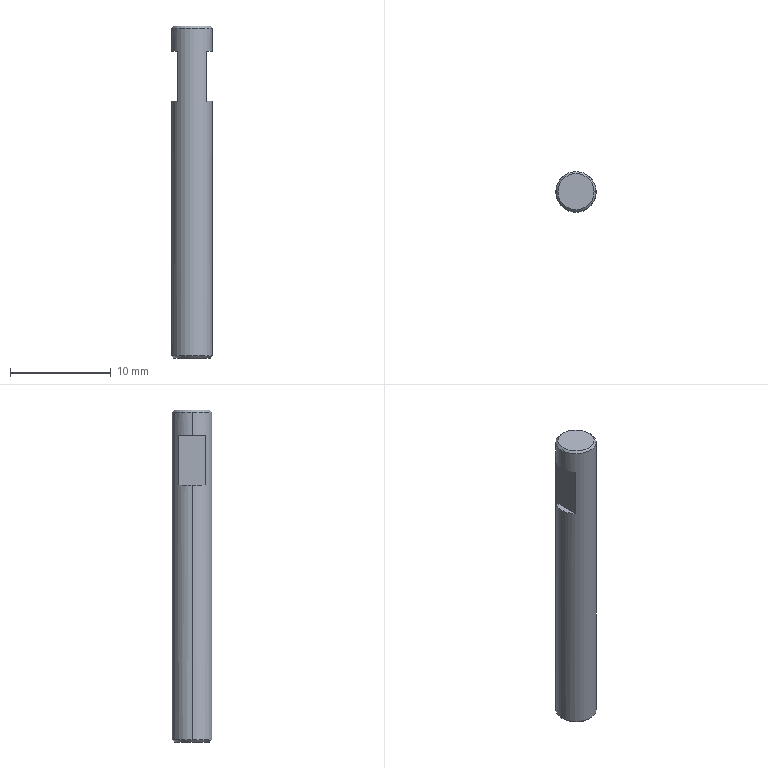Part | SolidWorks | features BaseBody 1, Chamfer 1 | 1 solid | 18 faces | box 4 x 4 x 33 mm | volume 382.151 mm3 | plane 8 | cone 6 | cylinder 4 | commonest cylinder face diameters 2.05 x2 4 x2
STEP:
#1=CARTESIAN_POINT('',(1.8,0.,16.5));
#2=VERTEX_POINT('',#1);
#3=CARTESIAN_POINT('',(-1.8,0.,16.5));
#4=VERTEX_POINT('',#3);
#5=CARTESIAN_POINT('',(0.,0.,16.5));
#6=DIRECTION('',(0.,0.,1.));
#7=DIRECTION('',(1.,0.,0.));
#8=AXIS2_PLACEMENT_3D('',#5,#6,#7);
#9=CIRCLE('',#8,1.8);
#10=EDGE_CURVE('',#2,#4,#9,.T.);
#11=ORIENTED_EDGE('',*,*,#10,.F.);
#12=CARTESIAN_POINT('',(2.,0.,16.3));
#13=VERTEX_POINT('',#12);
#14=CARTESIAN_POINT('',(2.,0.,16.3));
#15=DIRECTION('',(0.7071,0.,-0.7071));
#16=VECTOR('',#15,1000.);
#17=LINE('',#14,#16);
#18=EDGE_CURVE('',#2,#13,#17,.T.);
#19=ORIENTED_EDGE('',*,*,#18,.T.);
#20=CARTESIAN_POINT('',(-2.,0.,16.3));
#21=VERTEX_POINT('',#20);
#22=CARTESIAN_POINT('',(0.,0.,16.3));
#23=DIRECTION('',(0.,0.,-1.));
#24=DIRECTION('',(1.,0.,0.));
#25=AXIS2_PLACEMENT_3D('',#22,#23,#24);
#26=CIRCLE('',#25,2.);
#27=EDGE_CURVE('',#21,#13,#26,.T.);
#28=ORIENTED_EDGE('',*,*,#27,.F.);
#29=CARTESIAN_POINT('',(-2.,0.,16.3));
#30=DIRECTION('',(-0.7071,0.,-0.7071));
#31=VECTOR('',#30,1000.);
#32=LINE('',#29,#31);
#33=EDGE_CURVE('',#4,#21,#32,.T.);
#34=ORIENTED_EDGE('',*,*,#33,.F.);
#35=EDGE_LOOP('',(#11,#19,#28,#34));
#36=FACE_OUTER_BOUND('',#35,.T.);
#37=CARTESIAN_POINT('',(0.,0.,16.3));
#38=DIRECTION('',(0.,0.,-1.));
#39=DIRECTION('',(-1.,0.,0.));
#40=AXIS2_PLACEMENT_3D('',#37,#38,#39);
#41=CONICAL_SURFACE('',#40,2.,0.7854);
#42=ADVANCED_FACE('',(#36),#41,.T.);
#43=CARTESIAN_POINT('',(-1.8,0.,-16.5));
#44=VERTEX_POINT('',#43);
#45=CARTESIAN_POINT('',(1.8,0.,-16.5));
#46=VERTEX_POINT('',#45);
#47=CARTESIAN_POINT('',(0.,0.,-16.5));
#48=DIRECTION('',(0.,0.,-1.));
#49=DIRECTION('',(1.,0.,0.));
#50=AXIS2_PLACEMENT_3D('',#47,#48,#49);
#51=CIRCLE('',#50,1.8);
#52=EDGE_CURVE('',#44,#46,#51,.T.);
#53=ORIENTED_EDGE('',*,*,#52,.F.);
#54=CARTESIAN_POINT('',(-2.,0.,-16.3));
#55=VERTEX_POINT('',#54);
#56=CARTESIAN_POINT('',(-2.,0.,-16.3));
#57=DIRECTION('',(-0.7071,0.,0.7071));
#58=VECTOR('',#57,1000.);
#59=LINE('',#56,#58);
#60=EDGE_CURVE('',#44,#55,#59,.T.);
#61=ORIENTED_EDGE('',*,*,#60,.T.);
#62=CARTESIAN_POINT('',(2.,0.,-16.3));
#63=VERTEX_POINT('',#62);
#64=CARTESIAN_POINT('',(0.,0.,-16.3));
#65=DIRECTION('',(0.,0.,1.));
#66=DIRECTION('',(1.,0.,0.));
#67=AXIS2_PLACEMENT_3D('',#64,#65,#66);
#68=CIRCLE('',#67,2.);
#69=EDGE_CURVE('',#63,#55,#68,.T.);
#70=ORIENTED_EDGE('',*,*,#69,.F.);
#71=CARTESIAN_POINT('',(2.,0.,-16.3));
#72=DIRECTION('',(0.7071,0.,0.7071));
#73=VECTOR('',#72,1000.);
#74=LINE('',#71,#73);
#75=EDGE_CURVE('',#46,#63,#74,.T.);
#76=ORIENTED_EDGE('',*,*,#75,.F.);
#77=EDGE_LOOP('',(#53,#61,#70,#76));
#78=FACE_OUTER_BOUND('',#77,.T.);
#79=CARTESIAN_POINT('',(0.,0.,-16.3));
#80=DIRECTION('',(0.,0.,1.));
#81=DIRECTION('',(1.,0.,0.));
#82=AXIS2_PLACEMENT_3D('',#79,#80,#81);
#83=CONICAL_SURFACE('',#82,2.,0.7854);
#84=ADVANCED_FACE('',(#78),#83,.T.);
#85=ORIENTED_EDGE('',*,*,#27,.T.);
#86=CARTESIAN_POINT('',(2.,0.,14.));
#87=VERTEX_POINT('',#86);
#88=CARTESIAN_POINT('',(2.,0.,16.5));
#89=DIRECTION('',(0.,0.,-1.));
#90=VECTOR('',#89,1000.);
#91=LINE('',#88,#90);
#92=EDGE_CURVE('',#13,#87,#91,.T.);
#93=ORIENTED_EDGE('',*,*,#92,.T.);
#94=CARTESIAN_POINT('',(1.45,1.377,14.));
#95=VERTEX_POINT('',#94);
#96=CARTESIAN_POINT('',(0.,0.,14.));
#97=DIRECTION('',(0.,0.,1.));
#98=DIRECTION('',(-1.,0.,0.));
#99=AXIS2_PLACEMENT_3D('',#96,#97,#98);
#100=CIRCLE('',#99,2.);
#101=EDGE_CURVE('',#87,#95,#100,.T.);
#102=ORIENTED_EDGE('',*,*,#101,.T.);
#103=CARTESIAN_POINT('',(1.45,1.377,9.));
#104=VERTEX_POINT('',#103);
#105=CARTESIAN_POINT('',(1.45,1.377,16.5));
#106=DIRECTION('',(0.,0.,-1.));
#107=VECTOR('',#106,1000.);
#108=LINE('',#105,#107);
#109=EDGE_CURVE('',#95,#104,#108,.T.);
#110=ORIENTED_EDGE('',*,*,#109,.T.);
#111=CARTESIAN_POINT('',(2.,0.,9.));
#112=VERTEX_POINT('',#111);
#113=CARTESIAN_POINT('',(0.,0.,9.));
#114=DIRECTION('',(0.,0.,-1.));
#115=DIRECTION('',(-1.,0.,0.));
#116=AXIS2_PLACEMENT_3D('',#113,#114,#115);
#117=CIRCLE('',#116,2.);
#118=EDGE_CURVE('',#104,#112,#117,.T.);
#119=ORIENTED_EDGE('',*,*,#118,.T.);
#120=CARTESIAN_POINT('',(2.,0.,16.5));
#121=DIRECTION('',(0.,0.,-1.));
#122=VECTOR('',#121,1000.);
#123=LINE('',#120,#122);
#124=EDGE_CURVE('',#112,#63,#123,.T.);
#125=ORIENTED_EDGE('',*,*,#124,.T.);
#126=ORIENTED_EDGE('',*,*,#69,.T.);
#127=CARTESIAN_POINT('',(-2.,0.,9.));
#128=VERTEX_POINT('',#127);
#129=CARTESIAN_POINT('',(-2.,0.,16.5));
#130=DIRECTION('',(0.,0.,-1.));
#131=VECTOR('',#130,1000.);
#132=LINE('',#129,#131);
#133=EDGE_CURVE('',#128,#55,#132,.T.);
#134=ORIENTED_EDGE('',*,*,#133,.F.);
#135=CARTESIAN_POINT('',(-1.45,1.377,9.));
#136=VERTEX_POINT('',#135);
#137=CARTESIAN_POINT('',(0.,0.,9.));
#138=DIRECTION('',(0.,0.,-1.));
#139=DIRECTION('',(-1.,0.,0.));
#140=AXIS2_PLACEMENT_3D('',#137,#138,#139);
#141=CIRCLE('',#140,2.);
#142=EDGE_CURVE('',#128,#136,#141,.T.);
#143=ORIENTED_EDGE('',*,*,#142,.T.);
#144=CARTESIAN_POINT('',(-1.45,1.377,14.));
#145=VERTEX_POINT('',#144);
#146=CARTESIAN_POINT('',(-1.45,1.377,16.5));
#147=DIRECTION('',(0.,0.,1.));
#148=VECTOR('',#147,1000.);
#149=LINE('',#146,#148);
#150=EDGE_CURVE('',#136,#145,#149,.T.);
#151=ORIENTED_EDGE('',*,*,#150,.T.);
#152=CARTESIAN_POINT('',(-2.,0.,14.));
#153=VERTEX_POINT('',#152);
#154=CARTESIAN_POINT('',(0.,0.,14.));
#155=DIRECTION('',(0.,0.,1.));
#156=DIRECTION('',(-1.,0.,0.));
#157=AXIS2_PLACEMENT_3D('',#154,#155,#156);
#158=CIRCLE('',#157,2.);
#159=EDGE_CURVE('',#145,#153,#158,.T.);
#160=ORIENTED_EDGE('',*,*,#159,.T.);
#161=CARTESIAN_POINT('',(-2.,0.,16.5));
#162=DIRECTION('',(0.,0.,-1.));
#163=VECTOR('',#162,1000.);
#164=LINE('',#161,#163);
#165=EDGE_CURVE('',#21,#153,#164,.T.);
#166=ORIENTED_EDGE('',*,*,#165,.F.);
#167=EDGE_LOOP('',(#85,#93,#102,#110,#119,#125,#126,#134,#143,#151,#160,#166));
#168=FACE_OUTER_BOUND('',#167,.T.);
#169=CARTESIAN_POINT('',(0.,0.,16.5));
#170=DIRECTION('',(0.,0.,-1.));
#171=DIRECTION('',(-1.,0.,0.));
#172=AXIS2_PLACEMENT_3D('',#169,#170,#171);
#173=CYLINDRICAL_SURFACE('',#172,2.);
#174=ADVANCED_FACE('',(#168),#173,.T.);
#175=CARTESIAN_POINT('',(1.025,0.,-10.15));
#176=VERTEX_POINT('',#175);
#177=CARTESIAN_POINT('',(-1.025,0.,-10.15));
#178=VERTEX_POINT('',#177);
#179=CARTESIAN_POINT('',(0.,0.,-10.15));
#180=DIRECTION('',(0.,0.,-1.));
#181=DIRECTION('',(-1.,0.,0.));
#182=AXIS2_PLACEMENT_3D('',#179,#180,#181);
#183=CIRCLE('',#182,1.025);
#184=EDGE_CURVE('',#176,#178,#183,.T.);
#185=ORIENTED_EDGE('',*,*,#184,.F.);
#186=CARTESIAN_POINT('',(1.025,0.,-16.5));
#187=VERTEX_POINT('',#186);
#188=CARTESIAN_POINT('',(1.025,0.,-16.5));
#189=DIRECTION('',(0.,0.,-1.));
#190=VECTOR('',#189,1000.);
#191=LINE('',#188,#190);
#192=EDGE_CURVE('',#176,#187,#191,.T.);
#193=ORIENTED_EDGE('',*,*,#192,.T.);
#194=CARTESIAN_POINT('',(-1.025,0.,-16.5));
#195=VERTEX_POINT('',#194);
#196=CARTESIAN_POINT('',(0.,0.,-16.5));
#197=DIRECTION('',(0.,0.,-1.));
#198=DIRECTION('',(-1.,0.,0.));
#199=AXIS2_PLACEMENT_3D('',#196,#197,#198);
#200=CIRCLE('',#199,1.025);
#201=EDGE_CURVE('',#187,#195,#200,.T.);
#202=ORIENTED_EDGE('',*,*,#201,.T.);
#203=CARTESIAN_POINT('',(-1.025,0.,-16.5));
#204=DIRECTION('',(0.,0.,-1.));
#205=VECTOR('',#204,1000.);
#206=LINE('',#203,#205);
#207=EDGE_CURVE('',#178,#195,#206,.T.);
#208=ORIENTED_EDGE('',*,*,#207,.F.);
#209=EDGE_LOOP('',(#185,#193,#202,#208));
#210=FACE_OUTER_BOUND('',#209,.T.);
#211=CARTESIAN_POINT('',(0.,0.,-16.5));
#212=DIRECTION('',(0.,0.,-1.));
#213=DIRECTION('',(-1.,0.,0.));
#214=AXIS2_PLACEMENT_3D('',#211,#212,#213);
#215=CYLINDRICAL_SURFACE('',#214,1.025);
#216=ADVANCED_FACE('',(#210),#215,.F.);
#217=CARTESIAN_POINT('',(0.,0.,-9.534));
#218=VERTEX_POINT('',#217);
#219=CARTESIAN_POINT('',(-1.025,0.,-10.15));
#220=DIRECTION('',(-0.8572,0.,-0.515));
#221=VECTOR('',#220,1000.);
#222=LINE('',#219,#221);
#223=EDGE_CURVE('',#218,#178,#222,.T.);
#224=ORIENTED_EDGE('',*,*,#223,.F.);
#225=CARTESIAN_POINT('',(1.025,0.,-10.15));
#226=DIRECTION('',(0.8572,0.,-0.515));
#227=VECTOR('',#226,1000.);
#228=LINE('',#225,#227);
#229=EDGE_CURVE('',#218,#176,#228,.T.);
#230=ORIENTED_EDGE('',*,*,#229,.T.);
#231=ORIENTED_EDGE('',*,*,#184,.T.);
#232=EDGE_LOOP('',(#224,#230,#231));
#233=FACE_OUTER_BOUND('',#232,.T.);
#234=CARTESIAN_POINT('',(0.,0.,-10.15));
#235=DIRECTION('',(0.,0.,-1.));
#236=DIRECTION('',(-1.,0.,0.));
#237=AXIS2_PLACEMENT_3D('',#234,#235,#236);
#238=CONICAL_SURFACE('',#237,1.025,1.03);
#239=ADVANCED_FACE('',(#233),#238,.F.);
#240=ORIENTED_EDGE('',*,*,#92,.F.);
#241=CARTESIAN_POINT('',(0.,0.,16.3));
#242=DIRECTION('',(0.,0.,-1.));
#243=DIRECTION('',(1.,0.,0.));
#244=AXIS2_PLACEMENT_3D('',#241,#242,#243);
#245=CIRCLE('',#244,2.);
#246=EDGE_CURVE('',#13,#21,#245,.T.);
#247=ORIENTED_EDGE('',*,*,#246,.T.);
#248=ORIENTED_EDGE('',*,*,#165,.T.);
#249=CARTESIAN_POINT('',(-1.45,-1.377,14.));
#250=VERTEX_POINT('',#249);
#251=CARTESIAN_POINT('',(0.,0.,14.));
#252=DIRECTION('',(0.,0.,1.));
#253=DIRECTION('',(-1.,0.,0.));
#254=AXIS2_PLACEMENT_3D('',#251,#252,#253);
#255=CIRCLE('',#254,2.);
#256=EDGE_CURVE('',#153,#250,#255,.T.);
#257=ORIENTED_EDGE('',*,*,#256,.T.);
#258=CARTESIAN_POINT('',(-1.45,-1.377,9.));
#259=VERTEX_POINT('',#258);
#260=CARTESIAN_POINT('',(-1.45,-1.377,16.5));
#261=DIRECTION('',(0.,0.,-1.));
#262=VECTOR('',#261,1000.);
#263=LINE('',#260,#262);
#264=EDGE_CURVE('',#250,#259,#263,.T.);
#265=ORIENTED_EDGE('',*,*,#264,.T.);
#266=CARTESIAN_POINT('',(0.,0.,9.));
#267=DIRECTION('',(0.,0.,-1.));
#268=DIRECTION('',(-1.,0.,0.));
#269=AXIS2_PLACEMENT_3D('',#266,#267,#268);
#270=CIRCLE('',#269,2.);
#271=EDGE_CURVE('',#259,#128,#270,.T.);
#272=ORIENTED_EDGE('',*,*,#271,.T.);
#273=ORIENTED_EDGE('',*,*,#133,.T.);
#274=CARTESIAN_POINT('',(0.,0.,-16.3));
#275=DIRECTION('',(0.,0.,1.));
#276=DIRECTION('',(1.,0.,0.));
#277=AXIS2_PLACEMENT_3D('',#274,#275,#276);
#278=CIRCLE('',#277,2.);
#279=EDGE_CURVE('',#55,#63,#278,.T.);
#280=ORIENTED_EDGE('',*,*,#279,.T.);
#281=ORIENTED_EDGE('',*,*,#124,.F.);
#282=CARTESIAN_POINT('',(1.45,-1.377,9.));
#283=VERTEX_POINT('',#282);
#284=CARTESIAN_POINT('',(0.,0.,9.));
#285=DIRECTION('',(0.,0.,-1.));
#286=DIRECTION('',(-1.,0.,0.));
#287=AXIS2_PLACEMENT_3D('',#284,#285,#286);
#288=CIRCLE('',#287,2.);
#289=EDGE_CURVE('',#112,#283,#288,.T.);
#290=ORIENTED_EDGE('',*,*,#289,.T.);
#291=CARTESIAN_POINT('',(1.45,-1.377,14.));
#292=VERTEX_POINT('',#291);
#293=CARTESIAN_POINT('',(1.45,-1.377,16.5));
#294=DIRECTION('',(0.,0.,1.));
#295=VECTOR('',#294,1000.);
#296=LINE('',#293,#295);
#297=EDGE_CURVE('',#283,#292,#296,.T.);
#298=ORIENTED_EDGE('',*,*,#297,.T.);
#299=CARTESIAN_POINT('',(0.,0.,14.));
#300=DIRECTION('',(0.,0.,1.));
#301=DIRECTION('',(-1.,0.,0.));
#302=AXIS2_PLACEMENT_3D('',#299,#300,#301);
#303=CIRCLE('',#302,2.);
#304=EDGE_CURVE('',#292,#87,#303,.T.);
#305=ORIENTED_EDGE('',*,*,#304,.T.);
#306=EDGE_LOOP('',(#240,#247,#248,#257,#265,#272,#273,#280,#281,#290,#298,#305));
#307=FACE_OUTER_BOUND('',#306,.T.);
#308=CARTESIAN_POINT('',(0.,0.,16.5));
#309=DIRECTION('',(0.,0.,-1.));
#310=DIRECTION('',(-1.,0.,0.));
#311=AXIS2_PLACEMENT_3D('',#308,#309,#310);
#312=CYLINDRICAL_SURFACE('',#311,2.);
#313=ADVANCED_FACE('',(#307),#312,.T.);
#314=CARTESIAN_POINT('',(-1.45,-2.,14.));
#315=DIRECTION('',(0.,1.,0.));
#316=VECTOR('',#315,1000.);
#317=LINE('',#314,#316);
#318=EDGE_CURVE('',#250,#145,#317,.T.);
#319=ORIENTED_EDGE('',*,*,#318,.F.);
#320=ORIENTED_EDGE('',*,*,#256,.F.);
#321=ORIENTED_EDGE('',*,*,#159,.F.);
#322=EDGE_LOOP('',(#319,#320,#321));
#323=FACE_OUTER_BOUND('',#322,.T.);
#324=CARTESIAN_POINT('',(-2.,-2.,14.));
#325=DIRECTION('',(0.,0.,1.));
#326=DIRECTION('',(1.,0.,0.));
#327=AXIS2_PLACEMENT_3D('',#324,#325,#326);
#328=PLANE('',#327);
#329=ADVANCED_FACE('',(#323),#328,.F.);
#330=ORIENTED_EDGE('',*,*,#150,.F.);
#331=CARTESIAN_POINT('',(-1.45,-2.,9.));
#332=DIRECTION('',(0.,1.,0.));
#333=VECTOR('',#332,1000.);
#334=LINE('',#331,#333);
#335=EDGE_CURVE('',#259,#136,#334,.T.);
#336=ORIENTED_EDGE('',*,*,#335,.F.);
#337=ORIENTED_EDGE('',*,*,#264,.F.);
#338=ORIENTED_EDGE('',*,*,#318,.T.);
#339=EDGE_LOOP('',(#330,#336,#337,#338));
#340=FACE_OUTER_BOUND('',#339,.T.);
#341=CARTESIAN_POINT('',(-1.45,-2.,9.));
#342=DIRECTION('',(1.,0.,0.));
#343=DIRECTION('',(0.,0.,-1.));
#344=AXIS2_PLACEMENT_3D('',#341,#342,#343);
#345=PLANE('',#344);
#346=ADVANCED_FACE('',(#340),#345,.F.);
#347=ORIENTED_EDGE('',*,*,#335,.T.);
#348=ORIENTED_EDGE('',*,*,#142,.F.);
#349=ORIENTED_EDGE('',*,*,#271,.F.);
#350=EDGE_LOOP('',(#347,#348,#349));
#351=FACE_OUTER_BOUND('',#350,.T.);
#352=CARTESIAN_POINT('',(-2.,-2.,9.));
#353=DIRECTION('',(0.,0.,-1.));
#354=DIRECTION('',(-1.,0.,0.));
#355=AXIS2_PLACEMENT_3D('',#352,#353,#354);
#356=PLANE('',#355);
#357=ADVANCED_FACE('',(#351),#356,.F.);
#358=CARTESIAN_POINT('',(0.,0.,-16.5));
#359=DIRECTION('',(0.,0.,-1.));
#360=DIRECTION('',(1.,0.,0.));
#361=AXIS2_PLACEMENT_3D('',#358,#359,#360);
#362=CIRCLE('',#361,1.8);
#363=EDGE_CURVE('',#46,#44,#362,.T.);
#364=ORIENTED_EDGE('',*,*,#363,.T.);
#365=ORIENTED_EDGE('',*,*,#52,.T.);
#366=EDGE_LOOP('',(#364,#365));
#367=FACE_OUTER_BOUND('',#366,.T.);
#368=CARTESIAN_POINT('',(0.,0.,-16.5));
#369=DIRECTION('',(0.,0.,-1.));
#370=DIRECTION('',(-1.,0.,0.));
#371=AXIS2_PLACEMENT_3D('',#368,#369,#370);
#372=CIRCLE('',#371,1.025);
#373=EDGE_CURVE('',#195,#187,#372,.T.);
#374=ORIENTED_EDGE('',*,*,#373,.F.);
#375=ORIENTED_EDGE('',*,*,#201,.F.);
#376=EDGE_LOOP('',(#374,#375));
#377=FACE_BOUND('',#376,.T.);
#378=CARTESIAN_POINT('',(0.,0.,-16.5));
#379=DIRECTION('',(0.,0.,1.));
#380=DIRECTION('',(1.,0.,0.));
#381=AXIS2_PLACEMENT_3D('',#378,#379,#380);
#382=PLANE('',#381);
#383=ADVANCED_FACE('',(#367,#377),#382,.F.);
#384=ORIENTED_EDGE('',*,*,#118,.F.);
#385=CARTESIAN_POINT('',(1.45,-2.,9.));
#386=DIRECTION('',(0.,-1.,0.));
#387=VECTOR('',#386,1000.);
#388=LINE('',#385,#387);
#389=EDGE_CURVE('',#104,#283,#388,.T.);
#390=ORIENTED_EDGE('',*,*,#389,.T.);
#391=ORIENTED_EDGE('',*,*,#289,.F.);
#392=EDGE_LOOP('',(#384,#390,#391));
#393=FACE_OUTER_BOUND('',#392,.T.);
#394=CARTESIAN_POINT('',(2.,-2.,9.));
#395=DIRECTION('',(0.,0.,1.));
#396=DIRECTION('',(1.,0.,0.));
#397=AXIS2_PLACEMENT_3D('',#394,#395,#396);
#398=PLANE('',#397);
#399=ADVANCED_FACE('',(#393),#398,.T.);
#400=ORIENTED_EDGE('',*,*,#109,.F.);
#401=CARTESIAN_POINT('',(1.45,-2.,14.));
#402=DIRECTION('',(0.,-1.,0.));
#403=VECTOR('',#402,1000.);
#404=LINE('',#401,#403);
#405=EDGE_CURVE('',#95,#292,#404,.T.);
#406=ORIENTED_EDGE('',*,*,#405,.T.);
#407=ORIENTED_EDGE('',*,*,#297,.F.);
#408=ORIENTED_EDGE('',*,*,#389,.F.);
#409=EDGE_LOOP('',(#400,#406,#407,#408));
#410=FACE_OUTER_BOUND('',#409,.T.);
#411=CARTESIAN_POINT('',(1.45,-2.,9.));
#412=DIRECTION('',(1.,0.,0.));
#413=DIRECTION('',(0.,0.,-1.));
#414=AXIS2_PLACEMENT_3D('',#411,#412,#413);
#415=PLANE('',#414);
#416=ADVANCED_FACE('',(#410),#415,.T.);
#417=ORIENTED_EDGE('',*,*,#304,.F.);
#418=ORIENTED_EDGE('',*,*,#405,.F.);
#419=ORIENTED_EDGE('',*,*,#101,.F.);
#420=EDGE_LOOP('',(#417,#418,#419));
#421=FACE_OUTER_BOUND('',#420,.T.);
#422=CARTESIAN_POINT('',(2.,-2.,14.));
#423=DIRECTION('',(0.,0.,-1.));
#424=DIRECTION('',(-1.,0.,0.));
#425=AXIS2_PLACEMENT_3D('',#422,#423,#424);
#426=PLANE('',#425);
#427=ADVANCED_FACE('',(#421),#426,.T.);
#428=CARTESIAN_POINT('',(0.,0.,16.5));
#429=DIRECTION('',(0.,0.,1.));
#430=DIRECTION('',(1.,0.,0.));
#431=AXIS2_PLACEMENT_3D('',#428,#429,#430);
#432=CIRCLE('',#431,1.8);
#433=EDGE_CURVE('',#4,#2,#432,.T.);
#434=ORIENTED_EDGE('',*,*,#433,.T.);
#435=ORIENTED_EDGE('',*,*,#10,.T.);
#436=EDGE_LOOP('',(#434,#435));
#437=FACE_OUTER_BOUND('',#436,.T.);
#438=CARTESIAN_POINT('',(0.,0.,16.5));
#439=DIRECTION('',(0.,0.,1.));
#440=DIRECTION('',(1.,0.,0.));
#441=AXIS2_PLACEMENT_3D('',#438,#439,#440);
#442=PLANE('',#441);
#443=ADVANCED_FACE('',(#437),#442,.T.);
#444=ORIENTED_EDGE('',*,*,#192,.F.);
#445=CARTESIAN_POINT('',(0.,0.,-10.15));
#446=DIRECTION('',(0.,0.,-1.));
#447=DIRECTION('',(-1.,0.,0.));
#448=AXIS2_PLACEMENT_3D('',#445,#446,#447);
#449=CIRCLE('',#448,1.025);
#450=EDGE_CURVE('',#178,#176,#449,.T.);
#451=ORIENTED_EDGE('',*,*,#450,.F.);
#452=ORIENTED_EDGE('',*,*,#207,.T.);
#453=ORIENTED_EDGE('',*,*,#373,.T.);
#454=EDGE_LOOP('',(#444,#451,#452,#453));
#455=FACE_OUTER_BOUND('',#454,.T.);
#456=CARTESIAN_POINT('',(0.,0.,-16.5));
#457=DIRECTION('',(0.,0.,-1.));
#458=DIRECTION('',(-1.,0.,0.));
#459=AXIS2_PLACEMENT_3D('',#456,#457,#458);
#460=CYLINDRICAL_SURFACE('',#459,1.025);
#461=ADVANCED_FACE('',(#455),#460,.F.);
#462=ORIENTED_EDGE('',*,*,#229,.F.);
#463=ORIENTED_EDGE('',*,*,#223,.T.);
#464=ORIENTED_EDGE('',*,*,#450,.T.);
#465=EDGE_LOOP('',(#462,#463,#464));
#466=FACE_OUTER_BOUND('',#465,.T.);
#467=CARTESIAN_POINT('',(0.,0.,-10.15));
#468=DIRECTION('',(0.,0.,-1.));
#469=DIRECTION('',(-1.,0.,0.));
#470=AXIS2_PLACEMENT_3D('',#467,#468,#469);
#471=CONICAL_SURFACE('',#470,1.025,1.03);
#472=ADVANCED_FACE('',(#466),#471,.F.);
#473=ORIENTED_EDGE('',*,*,#60,.F.);
#474=ORIENTED_EDGE('',*,*,#363,.F.);
#475=ORIENTED_EDGE('',*,*,#75,.T.);
#476=ORIENTED_EDGE('',*,*,#279,.F.);
#477=EDGE_LOOP('',(#473,#474,#475,#476));
#478=FACE_OUTER_BOUND('',#477,.T.);
#479=CARTESIAN_POINT('',(0.,0.,-16.3));
#480=DIRECTION('',(0.,0.,1.));
#481=DIRECTION('',(1.,0.,0.));
#482=AXIS2_PLACEMENT_3D('',#479,#480,#481);
#483=CONICAL_SURFACE('',#482,2.,0.7854);
#484=ADVANCED_FACE('',(#478),#483,.T.);
#485=ORIENTED_EDGE('',*,*,#18,.F.);
#486=ORIENTED_EDGE('',*,*,#433,.F.);
#487=ORIENTED_EDGE('',*,*,#33,.T.);
#488=ORIENTED_EDGE('',*,*,#246,.F.);
#489=EDGE_LOOP('',(#485,#486,#487,#488));
#490=FACE_OUTER_BOUND('',#489,.T.);
#491=CARTESIAN_POINT('',(0.,0.,16.3));
#492=DIRECTION('',(0.,0.,-1.));
#493=DIRECTION('',(-1.,0.,0.));
#494=AXIS2_PLACEMENT_3D('',#491,#492,#493);
#495=CONICAL_SURFACE('',#494,2.,0.7854);
#496=ADVANCED_FACE('',(#490),#495,.T.);
#497=CLOSED_SHELL('',(#42,#84,#174,#216,#239,#313,#329,#346,#357,#383,#399,#416,#427,#443,#461,#472,#484,#496));
#498=MANIFOLD_SOLID_BREP('',#497);
#499=CARTESIAN_POINT('',(0.,0.,0.));
#500=DIRECTION('',(0.,0.,1.));
#501=DIRECTION('',(1.,0.,0.));
#502=AXIS2_PLACEMENT_3D('',#499,#500,#501);
#503=(LENGTH_UNIT()NAMED_UNIT(*)SI_UNIT(.MILLI.,.METRE.));
#504=UNCERTAINTY_MEASURE_WITH_UNIT(LENGTH_MEASURE(0.00001),#503,'','');
#505=(NAMED_UNIT(*)PLANE_ANGLE_UNIT()SI_UNIT($,.RADIAN.));
#506=(NAMED_UNIT(*)SI_UNIT($,.STERADIAN.)SOLID_ANGLE_UNIT());
#507=(GEOMETRIC_REPRESENTATION_CONTEXT(3)GLOBAL_UNCERTAINTY_ASSIGNED_CONTEXT((#504))GLOBAL_UNIT_ASSIGNED_CONTEXT((#503,#505,#506))REPRESENTATION_CONTEXT('',''));
#508=ADVANCED_BREP_SHAPE_REPRESENTATION('',(#498,#502),#507);